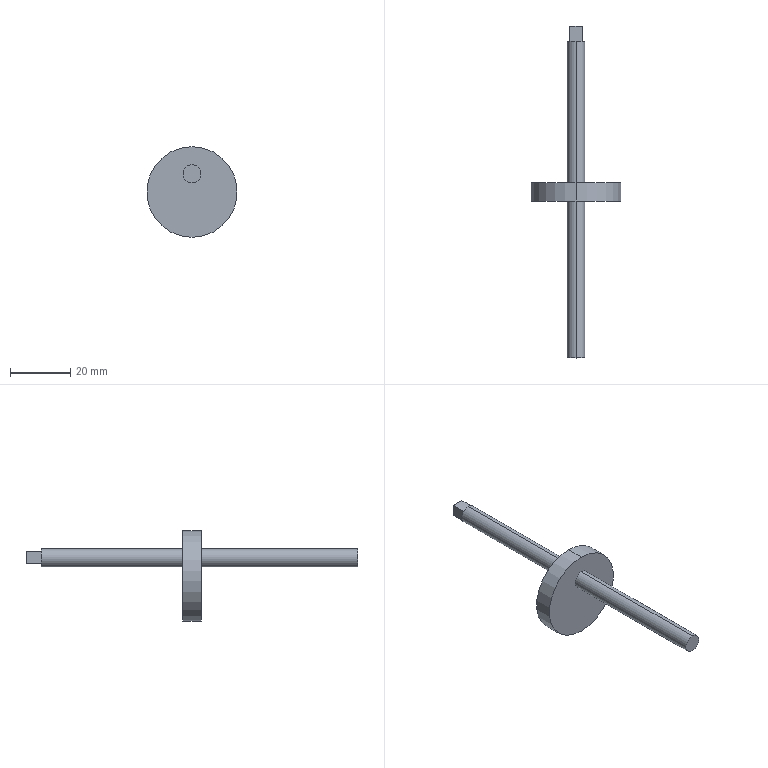Part | SolidWorks | features ICE 2, Extrusion 1 | 1 solid | 15 faces | box 30 x 110 x 30 mm | volume 7120 mm3 | plane 9 | cylinder 6 | commonest cylinder face diameters 6 x4 30 x2
STEP:
#1=CARTESIAN_POINT('',(0.,-3.,3.));
#2=VERTEX_POINT('',#1);
#3=CARTESIAN_POINT('',(0.,-3.,9.));
#4=VERTEX_POINT('',#3);
#5=CARTESIAN_POINT('',(0.,-3.,6.));
#6=DIRECTION('',(0.,-1.,0.));
#7=DIRECTION('',(0.,0.,1.));
#8=AXIS2_PLACEMENT_3D('',#5,#6,#7);
#9=CIRCLE('',#8,3.);
#10=EDGE_CURVE('',#2,#4,#9,.T.);
#11=ORIENTED_EDGE('',*,*,#10,.T.);
#12=CARTESIAN_POINT('',(0.,-55.,9.));
#13=VERTEX_POINT('',#12);
#14=CARTESIAN_POINT('',(0.,55.,9.));
#15=DIRECTION('',(0.,-1.,0.));
#16=VECTOR('',#15,1000.);
#17=LINE('',#14,#16);
#18=EDGE_CURVE('',#4,#13,#17,.T.);
#19=ORIENTED_EDGE('',*,*,#18,.T.);
#20=CARTESIAN_POINT('',(0.,-55.,3.));
#21=VERTEX_POINT('',#20);
#22=CARTESIAN_POINT('',(0.,-55.,6.));
#23=DIRECTION('',(0.,1.,0.));
#24=DIRECTION('',(0.,0.,1.));
#25=AXIS2_PLACEMENT_3D('',#22,#23,#24);
#26=CIRCLE('',#25,3.);
#27=EDGE_CURVE('',#13,#21,#26,.T.);
#28=ORIENTED_EDGE('',*,*,#27,.T.);
#29=CARTESIAN_POINT('',(0.,55.,3.));
#30=DIRECTION('',(0.,-1.,0.));
#31=VECTOR('',#30,1000.);
#32=LINE('',#29,#31);
#33=EDGE_CURVE('',#2,#21,#32,.T.);
#34=ORIENTED_EDGE('',*,*,#33,.F.);
#35=EDGE_LOOP('',(#11,#19,#28,#34));
#36=FACE_OUTER_BOUND('',#35,.T.);
#37=CARTESIAN_POINT('',(0.,55.,6.));
#38=DIRECTION('',(0.,-1.,0.));
#39=DIRECTION('',(0.,0.,-1.));
#40=AXIS2_PLACEMENT_3D('',#37,#38,#39);
#41=CYLINDRICAL_SURFACE('',#40,3.);
#42=ADVANCED_FACE('',(#36),#41,.T.);
#43=CARTESIAN_POINT('',(0.,3.,15.));
#44=VERTEX_POINT('',#43);
#45=CARTESIAN_POINT('',(0.,3.,-15.));
#46=VERTEX_POINT('',#45);
#47=CARTESIAN_POINT('',(0.,3.,0.));
#48=DIRECTION('',(0.,1.,0.));
#49=DIRECTION('',(0.,0.,1.));
#50=AXIS2_PLACEMENT_3D('',#47,#48,#49);
#51=CIRCLE('',#50,15.);
#52=EDGE_CURVE('',#44,#46,#51,.T.);
#53=ORIENTED_EDGE('',*,*,#52,.F.);
#54=CARTESIAN_POINT('',(0.,-3.,15.));
#55=VERTEX_POINT('',#54);
#56=CARTESIAN_POINT('',(0.,3.,15.));
#57=DIRECTION('',(0.,-1.,0.));
#58=VECTOR('',#57,1000.);
#59=LINE('',#56,#58);
#60=EDGE_CURVE('',#44,#55,#59,.T.);
#61=ORIENTED_EDGE('',*,*,#60,.T.);
#62=CARTESIAN_POINT('',(0.,-3.,-15.));
#63=VERTEX_POINT('',#62);
#64=CARTESIAN_POINT('',(0.,-3.,0.));
#65=DIRECTION('',(0.,1.,0.));
#66=DIRECTION('',(0.,0.,1.));
#67=AXIS2_PLACEMENT_3D('',#64,#65,#66);
#68=CIRCLE('',#67,15.);
#69=EDGE_CURVE('',#55,#63,#68,.T.);
#70=ORIENTED_EDGE('',*,*,#69,.T.);
#71=CARTESIAN_POINT('',(0.,3.,-15.));
#72=DIRECTION('',(0.,-1.,0.));
#73=VECTOR('',#72,1000.);
#74=LINE('',#71,#73);
#75=EDGE_CURVE('',#46,#63,#74,.T.);
#76=ORIENTED_EDGE('',*,*,#75,.F.);
#77=EDGE_LOOP('',(#53,#61,#70,#76));
#78=FACE_OUTER_BOUND('',#77,.T.);
#79=CARTESIAN_POINT('',(0.,3.,0.));
#80=DIRECTION('',(0.,-1.,0.));
#81=DIRECTION('',(0.,0.,-1.));
#82=AXIS2_PLACEMENT_3D('',#79,#80,#81);
#83=CYLINDRICAL_SURFACE('',#82,15.);
#84=ADVANCED_FACE('',(#78),#83,.T.);
#85=CARTESIAN_POINT('',(0.,50.,9.));
#86=VERTEX_POINT('',#85);
#87=CARTESIAN_POINT('',(0.,50.,3.));
#88=VERTEX_POINT('',#87);
#89=CARTESIAN_POINT('',(0.,50.,6.));
#90=DIRECTION('',(0.,1.,0.));
#91=DIRECTION('',(0.,0.,1.));
#92=AXIS2_PLACEMENT_3D('',#89,#90,#91);
#93=CIRCLE('',#92,3.);
#94=EDGE_CURVE('',#86,#88,#93,.T.);
#95=ORIENTED_EDGE('',*,*,#94,.F.);
#96=CARTESIAN_POINT('',(0.,3.,9.));
#97=VERTEX_POINT('',#96);
#98=CARTESIAN_POINT('',(0.,55.,9.));
#99=DIRECTION('',(0.,-1.,0.));
#100=VECTOR('',#99,1000.);
#101=LINE('',#98,#100);
#102=EDGE_CURVE('',#86,#97,#101,.T.);
#103=ORIENTED_EDGE('',*,*,#102,.T.);
#104=CARTESIAN_POINT('',(0.,3.,3.));
#105=VERTEX_POINT('',#104);
#106=CARTESIAN_POINT('',(0.,3.,6.));
#107=DIRECTION('',(0.,-1.,0.));
#108=DIRECTION('',(0.,0.,1.));
#109=AXIS2_PLACEMENT_3D('',#106,#107,#108);
#110=CIRCLE('',#109,3.);
#111=EDGE_CURVE('',#105,#97,#110,.T.);
#112=ORIENTED_EDGE('',*,*,#111,.F.);
#113=CARTESIAN_POINT('',(0.,55.,3.));
#114=DIRECTION('',(0.,-1.,0.));
#115=VECTOR('',#114,1000.);
#116=LINE('',#113,#115);
#117=EDGE_CURVE('',#88,#105,#116,.T.);
#118=ORIENTED_EDGE('',*,*,#117,.F.);
#119=EDGE_LOOP('',(#95,#103,#112,#118));
#120=FACE_OUTER_BOUND('',#119,.T.);
#121=CARTESIAN_POINT('',(0.,55.,6.));
#122=DIRECTION('',(0.,-1.,0.));
#123=DIRECTION('',(0.,0.,-1.));
#124=AXIS2_PLACEMENT_3D('',#121,#122,#123);
#125=CYLINDRICAL_SURFACE('',#124,3.);
#126=ADVANCED_FACE('',(#120),#125,.T.);
#127=ORIENTED_EDGE('',*,*,#102,.F.);
#128=CARTESIAN_POINT('',(0.,50.,6.));
#129=DIRECTION('',(0.,1.,0.));
#130=DIRECTION('',(0.,0.,1.));
#131=AXIS2_PLACEMENT_3D('',#128,#129,#130);
#132=CIRCLE('',#131,3.);
#133=EDGE_CURVE('',#88,#86,#132,.T.);
#134=ORIENTED_EDGE('',*,*,#133,.F.);
#135=ORIENTED_EDGE('',*,*,#117,.T.);
#136=CARTESIAN_POINT('',(0.,3.,6.));
#137=DIRECTION('',(0.,-1.,0.));
#138=DIRECTION('',(0.,0.,1.));
#139=AXIS2_PLACEMENT_3D('',#136,#137,#138);
#140=CIRCLE('',#139,3.);
#141=EDGE_CURVE('',#97,#105,#140,.T.);
#142=ORIENTED_EDGE('',*,*,#141,.F.);
#143=EDGE_LOOP('',(#127,#134,#135,#142));
#144=FACE_OUTER_BOUND('',#143,.T.);
#145=CARTESIAN_POINT('',(0.,55.,6.));
#146=DIRECTION('',(0.,-1.,0.));
#147=DIRECTION('',(0.,0.,-1.));
#148=AXIS2_PLACEMENT_3D('',#145,#146,#147);
#149=CYLINDRICAL_SURFACE('',#148,3.);
#150=ADVANCED_FACE('',(#144),#149,.T.);
#151=ORIENTED_EDGE('',*,*,#60,.F.);
#152=CARTESIAN_POINT('',(0.,3.,0.));
#153=DIRECTION('',(0.,1.,0.));
#154=DIRECTION('',(0.,0.,1.));
#155=AXIS2_PLACEMENT_3D('',#152,#153,#154);
#156=CIRCLE('',#155,15.);
#157=EDGE_CURVE('',#46,#44,#156,.T.);
#158=ORIENTED_EDGE('',*,*,#157,.F.);
#159=ORIENTED_EDGE('',*,*,#75,.T.);
#160=CARTESIAN_POINT('',(0.,-3.,0.));
#161=DIRECTION('',(0.,1.,0.));
#162=DIRECTION('',(0.,0.,1.));
#163=AXIS2_PLACEMENT_3D('',#160,#161,#162);
#164=CIRCLE('',#163,15.);
#165=EDGE_CURVE('',#63,#55,#164,.T.);
#166=ORIENTED_EDGE('',*,*,#165,.T.);
#167=EDGE_LOOP('',(#151,#158,#159,#166));
#168=FACE_OUTER_BOUND('',#167,.T.);
#169=CARTESIAN_POINT('',(0.,3.,0.));
#170=DIRECTION('',(0.,-1.,0.));
#171=DIRECTION('',(0.,0.,-1.));
#172=AXIS2_PLACEMENT_3D('',#169,#170,#171);
#173=CYLINDRICAL_SURFACE('',#172,15.);
#174=ADVANCED_FACE('',(#168),#173,.T.);
#175=ORIENTED_EDGE('',*,*,#111,.T.);
#176=ORIENTED_EDGE('',*,*,#141,.T.);
#177=EDGE_LOOP('',(#175,#176));
#178=FACE_BOUND('',#177,.T.);
#179=ORIENTED_EDGE('',*,*,#157,.T.);
#180=ORIENTED_EDGE('',*,*,#52,.T.);
#181=EDGE_LOOP('',(#179,#180));
#182=FACE_OUTER_BOUND('',#181,.T.);
#183=CARTESIAN_POINT('',(0.,3.,0.));
#184=DIRECTION('',(0.,1.,0.));
#185=DIRECTION('',(0.,0.,1.));
#186=AXIS2_PLACEMENT_3D('',#183,#184,#185);
#187=PLANE('',#186);
#188=ADVANCED_FACE('',(#178,#182),#187,.T.);
#189=ORIENTED_EDGE('',*,*,#10,.F.);
#190=CARTESIAN_POINT('',(0.,-3.,6.));
#191=DIRECTION('',(0.,-1.,0.));
#192=DIRECTION('',(0.,0.,1.));
#193=AXIS2_PLACEMENT_3D('',#190,#191,#192);
#194=CIRCLE('',#193,3.);
#195=EDGE_CURVE('',#4,#2,#194,.T.);
#196=ORIENTED_EDGE('',*,*,#195,.F.);
#197=EDGE_LOOP('',(#189,#196));
#198=FACE_BOUND('',#197,.T.);
#199=ORIENTED_EDGE('',*,*,#165,.F.);
#200=ORIENTED_EDGE('',*,*,#69,.F.);
#201=EDGE_LOOP('',(#199,#200));
#202=FACE_OUTER_BOUND('',#201,.T.);
#203=CARTESIAN_POINT('',(0.,-3.,0.));
#204=DIRECTION('',(0.,1.,0.));
#205=DIRECTION('',(0.,0.,1.));
#206=AXIS2_PLACEMENT_3D('',#203,#204,#205);
#207=PLANE('',#206);
#208=ADVANCED_FACE('',(#198,#202),#207,.F.);
#209=CARTESIAN_POINT('',(0.,-55.,6.));
#210=DIRECTION('',(0.,1.,0.));
#211=DIRECTION('',(0.,0.,1.));
#212=AXIS2_PLACEMENT_3D('',#209,#210,#211);
#213=CIRCLE('',#212,3.);
#214=EDGE_CURVE('',#21,#13,#213,.T.);
#215=ORIENTED_EDGE('',*,*,#214,.F.);
#216=ORIENTED_EDGE('',*,*,#27,.F.);
#217=EDGE_LOOP('',(#215,#216));
#218=FACE_OUTER_BOUND('',#217,.T.);
#219=CARTESIAN_POINT('',(0.,-55.,6.));
#220=DIRECTION('',(0.,1.,0.));
#221=DIRECTION('',(0.,0.,1.));
#222=AXIS2_PLACEMENT_3D('',#219,#220,#221);
#223=PLANE('',#222);
#224=ADVANCED_FACE('',(#218),#223,.F.);
#225=ORIENTED_EDGE('',*,*,#18,.F.);
#226=ORIENTED_EDGE('',*,*,#195,.T.);
#227=ORIENTED_EDGE('',*,*,#33,.T.);
#228=ORIENTED_EDGE('',*,*,#214,.T.);
#229=EDGE_LOOP('',(#225,#226,#227,#228));
#230=FACE_OUTER_BOUND('',#229,.T.);
#231=CARTESIAN_POINT('',(0.,55.,6.));
#232=DIRECTION('',(0.,-1.,0.));
#233=DIRECTION('',(0.,0.,-1.));
#234=AXIS2_PLACEMENT_3D('',#231,#232,#233);
#235=CYLINDRICAL_SURFACE('',#234,3.);
#236=ADVANCED_FACE('',(#230),#235,.T.);
#237=CARTESIAN_POINT('',(-2.,50.,8.));
#238=VERTEX_POINT('',#237);
#239=CARTESIAN_POINT('',(2.,50.,8.));
#240=VERTEX_POINT('',#239);
#241=CARTESIAN_POINT('',(-2.,50.,8.));
#242=DIRECTION('',(1.,0.,0.));
#243=VECTOR('',#242,1000.);
#244=LINE('',#241,#243);
#245=EDGE_CURVE('',#238,#240,#244,.T.);
#246=ORIENTED_EDGE('',*,*,#245,.F.);
#247=CARTESIAN_POINT('',(-2.,50.,4.));
#248=VERTEX_POINT('',#247);
#249=CARTESIAN_POINT('',(-2.,50.,8.));
#250=DIRECTION('',(0.,0.,1.));
#251=VECTOR('',#250,1000.);
#252=LINE('',#249,#251);
#253=EDGE_CURVE('',#248,#238,#252,.T.);
#254=ORIENTED_EDGE('',*,*,#253,.F.);
#255=CARTESIAN_POINT('',(2.,50.,4.));
#256=VERTEX_POINT('',#255);
#257=CARTESIAN_POINT('',(-2.,50.,4.));
#258=DIRECTION('',(-1.,0.,0.));
#259=VECTOR('',#258,1000.);
#260=LINE('',#257,#259);
#261=EDGE_CURVE('',#256,#248,#260,.T.);
#262=ORIENTED_EDGE('',*,*,#261,.F.);
#263=CARTESIAN_POINT('',(2.,50.,8.));
#264=DIRECTION('',(0.,0.,-1.));
#265=VECTOR('',#264,1000.);
#266=LINE('',#263,#265);
#267=EDGE_CURVE('',#240,#256,#266,.T.);
#268=ORIENTED_EDGE('',*,*,#267,.F.);
#269=EDGE_LOOP('',(#246,#254,#262,#268));
#270=FACE_BOUND('',#269,.T.);
#271=ORIENTED_EDGE('',*,*,#133,.T.);
#272=ORIENTED_EDGE('',*,*,#94,.T.);
#273=EDGE_LOOP('',(#271,#272));
#274=FACE_OUTER_BOUND('',#273,.T.);
#275=CARTESIAN_POINT('',(0.,50.,6.));
#276=DIRECTION('',(0.,1.,0.));
#277=DIRECTION('',(0.,0.,1.));
#278=AXIS2_PLACEMENT_3D('',#275,#276,#277);
#279=PLANE('',#278);
#280=ADVANCED_FACE('',(#270,#274),#279,.T.);
#281=CARTESIAN_POINT('',(2.,55.,8.));
#282=VERTEX_POINT('',#281);
#283=CARTESIAN_POINT('',(2.,55.,4.));
#284=VERTEX_POINT('',#283);
#285=CARTESIAN_POINT('',(2.,55.,8.));
#286=DIRECTION('',(0.,0.,-1.));
#287=VECTOR('',#286,1000.);
#288=LINE('',#285,#287);
#289=EDGE_CURVE('',#282,#284,#288,.T.);
#290=ORIENTED_EDGE('',*,*,#289,.F.);
#291=CARTESIAN_POINT('',(2.,50.,8.));
#292=DIRECTION('',(0.,1.,0.));
#293=VECTOR('',#292,1000.);
#294=LINE('',#291,#293);
#295=EDGE_CURVE('',#240,#282,#294,.T.);
#296=ORIENTED_EDGE('',*,*,#295,.F.);
#297=ORIENTED_EDGE('',*,*,#267,.T.);
#298=CARTESIAN_POINT('',(2.,50.,4.));
#299=DIRECTION('',(0.,1.,0.));
#300=VECTOR('',#299,1000.);
#301=LINE('',#298,#300);
#302=EDGE_CURVE('',#256,#284,#301,.T.);
#303=ORIENTED_EDGE('',*,*,#302,.T.);
#304=EDGE_LOOP('',(#290,#296,#297,#303));
#305=FACE_OUTER_BOUND('',#304,.T.);
#306=CARTESIAN_POINT('',(2.,50.,8.));
#307=DIRECTION('',(1.,0.,0.));
#308=DIRECTION('',(0.,0.,-1.));
#309=AXIS2_PLACEMENT_3D('',#306,#307,#308);
#310=PLANE('',#309);
#311=ADVANCED_FACE('',(#305),#310,.T.);
#312=CARTESIAN_POINT('',(-2.,55.,8.));
#313=VERTEX_POINT('',#312);
#314=CARTESIAN_POINT('',(-2.,55.,8.));
#315=DIRECTION('',(1.,0.,0.));
#316=VECTOR('',#315,1000.);
#317=LINE('',#314,#316);
#318=EDGE_CURVE('',#313,#282,#317,.T.);
#319=ORIENTED_EDGE('',*,*,#318,.F.);
#320=CARTESIAN_POINT('',(-2.,50.,8.));
#321=DIRECTION('',(0.,1.,0.));
#322=VECTOR('',#321,1000.);
#323=LINE('',#320,#322);
#324=EDGE_CURVE('',#238,#313,#323,.T.);
#325=ORIENTED_EDGE('',*,*,#324,.F.);
#326=ORIENTED_EDGE('',*,*,#245,.T.);
#327=ORIENTED_EDGE('',*,*,#295,.T.);
#328=EDGE_LOOP('',(#319,#325,#326,#327));
#329=FACE_OUTER_BOUND('',#328,.T.);
#330=CARTESIAN_POINT('',(-2.,50.,8.));
#331=DIRECTION('',(0.,0.,1.));
#332=DIRECTION('',(1.,0.,0.));
#333=AXIS2_PLACEMENT_3D('',#330,#331,#332);
#334=PLANE('',#333);
#335=ADVANCED_FACE('',(#329),#334,.T.);
#336=CARTESIAN_POINT('',(-2.,55.,4.));
#337=VERTEX_POINT('',#336);
#338=CARTESIAN_POINT('',(-2.,55.,8.));
#339=DIRECTION('',(0.,0.,1.));
#340=VECTOR('',#339,1000.);
#341=LINE('',#338,#340);
#342=EDGE_CURVE('',#337,#313,#341,.T.);
#343=ORIENTED_EDGE('',*,*,#342,.F.);
#344=CARTESIAN_POINT('',(-2.,50.,4.));
#345=DIRECTION('',(0.,1.,0.));
#346=VECTOR('',#345,1000.);
#347=LINE('',#344,#346);
#348=EDGE_CURVE('',#248,#337,#347,.T.);
#349=ORIENTED_EDGE('',*,*,#348,.F.);
#350=ORIENTED_EDGE('',*,*,#253,.T.);
#351=ORIENTED_EDGE('',*,*,#324,.T.);
#352=EDGE_LOOP('',(#343,#349,#350,#351));
#353=FACE_OUTER_BOUND('',#352,.T.);
#354=CARTESIAN_POINT('',(-2.,50.,8.));
#355=DIRECTION('',(-1.,0.,0.));
#356=DIRECTION('',(0.,0.,1.));
#357=AXIS2_PLACEMENT_3D('',#354,#355,#356);
#358=PLANE('',#357);
#359=ADVANCED_FACE('',(#353),#358,.T.);
#360=CARTESIAN_POINT('',(-2.,55.,4.));
#361=DIRECTION('',(-1.,0.,0.));
#362=VECTOR('',#361,1000.);
#363=LINE('',#360,#362);
#364=EDGE_CURVE('',#284,#337,#363,.T.);
#365=ORIENTED_EDGE('',*,*,#364,.F.);
#366=ORIENTED_EDGE('',*,*,#302,.F.);
#367=ORIENTED_EDGE('',*,*,#261,.T.);
#368=ORIENTED_EDGE('',*,*,#348,.T.);
#369=EDGE_LOOP('',(#365,#366,#367,#368));
#370=FACE_OUTER_BOUND('',#369,.T.);
#371=CARTESIAN_POINT('',(-2.,50.,4.));
#372=DIRECTION('',(0.,0.,-1.));
#373=DIRECTION('',(-1.,0.,0.));
#374=AXIS2_PLACEMENT_3D('',#371,#372,#373);
#375=PLANE('',#374);
#376=ADVANCED_FACE('',(#370),#375,.T.);
#377=ORIENTED_EDGE('',*,*,#318,.T.);
#378=ORIENTED_EDGE('',*,*,#289,.T.);
#379=ORIENTED_EDGE('',*,*,#364,.T.);
#380=ORIENTED_EDGE('',*,*,#342,.T.);
#381=EDGE_LOOP('',(#377,#378,#379,#380));
#382=FACE_OUTER_BOUND('',#381,.T.);
#383=CARTESIAN_POINT('',(0.,55.,6.));
#384=DIRECTION('',(0.,1.,0.));
#385=DIRECTION('',(0.,0.,1.));
#386=AXIS2_PLACEMENT_3D('',#383,#384,#385);
#387=PLANE('',#386);
#388=ADVANCED_FACE('',(#382),#387,.T.);
#389=CLOSED_SHELL('',(#42,#84,#126,#150,#174,#188,#208,#224,#236,#280,#311,#335,#359,#376,#388));
#390=MANIFOLD_SOLID_BREP('',#389);
#391=CARTESIAN_POINT('',(0.,0.,0.));
#392=DIRECTION('',(0.,0.,1.));
#393=DIRECTION('',(1.,0.,0.));
#394=AXIS2_PLACEMENT_3D('',#391,#392,#393);
#395=(LENGTH_UNIT()NAMED_UNIT(*)SI_UNIT(.MILLI.,.METRE.));
#396=UNCERTAINTY_MEASURE_WITH_UNIT(LENGTH_MEASURE(0.00001),#395,'','');
#397=(NAMED_UNIT(*)PLANE_ANGLE_UNIT()SI_UNIT($,.RADIAN.));
#398=(NAMED_UNIT(*)SI_UNIT($,.STERADIAN.)SOLID_ANGLE_UNIT());
#399=(GEOMETRIC_REPRESENTATION_CONTEXT(3)GLOBAL_UNCERTAINTY_ASSIGNED_CONTEXT((#396))GLOBAL_UNIT_ASSIGNED_CONTEXT((#395,#397,#398))REPRESENTATION_CONTEXT('',''));
#400=ADVANCED_BREP_SHAPE_REPRESENTATION('',(#390,#394),#399);